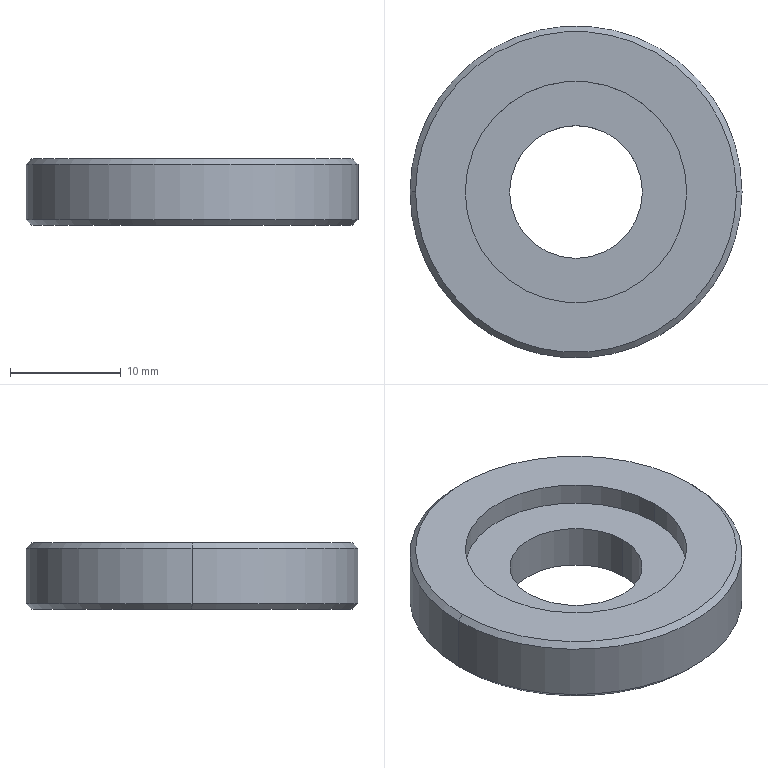Part | STEP file | PN_0100 Mount electronic clip blade | 1 solid | 13 faces | box 30 x 30 x 6 mm | volume 3137 mm3 | cylinder 6 | cone 4 | plane 3 | commonest cylinder face diameters 12 x2 20 x2 30 x2
STEP:
#1=CARTESIAN_POINT('',(0.,0.,0.));
#2=DIRECTION('',(0.,0.,1.));
#3=DIRECTION('',(1.,0.,0.));
#4=AXIS2_PLACEMENT_3D('',#1,#2,#3);
#5=CARTESIAN_POINT('',(14.5,0.,6.));
#6=VERTEX_POINT('',#5);
#7=CARTESIAN_POINT('',(-14.5,0.,6.));
#8=VERTEX_POINT('',#7);
#9=CARTESIAN_POINT('',(0.,0.,6.));
#10=DIRECTION('',(0.,0.,1.));
#11=DIRECTION('',(1.,0.,0.));
#12=AXIS2_PLACEMENT_3D('',#9,#10,#11);
#13=CIRCLE('',#12,14.5);
#14=CARTESIAN_POINT('',(0.,0.,6.));
#15=DIRECTION('',(0.,0.,-1.));
#16=DIRECTION('',(-1.,0.,0.));
#17=AXIS2_PLACEMENT_3D('',#14,#15,#16);
#18=CONICAL_SURFACE('',#17,14.5,0.7854);
#19=CARTESIAN_POINT('',(3.142,0.));
#20=DIRECTION('',(-1.,0.));
#21=VECTOR('',#20,1.);
#22=LINE('',#19,#21);
#23=(GEOMETRIC_REPRESENTATION_CONTEXT(2)PARAMETRIC_REPRESENTATION_CONTEXT()REPRESENTATION_CONTEXT('',''));
#24=DEFINITIONAL_REPRESENTATION('',(#22),#23);
#25=PCURVE('',#18,#24);
#26=CARTESIAN_POINT('',(0.,0.,6.));
#27=DIRECTION('',(0.,0.,1.));
#28=DIRECTION('',(1.,0.,0.));
#29=AXIS2_PLACEMENT_3D('',#26,#27,#28);
#30=PLANE('',#29);
#31=CARTESIAN_POINT('',(0.,0.));
#32=DIRECTION('',(1.,0.));
#33=AXIS2_PLACEMENT_2D('',#31,#32);
#34=CIRCLE('',#33,14.5);
#35=(GEOMETRIC_REPRESENTATION_CONTEXT(2)PARAMETRIC_REPRESENTATION_CONTEXT()REPRESENTATION_CONTEXT('',''));
#36=DEFINITIONAL_REPRESENTATION('',(#34),#35);
#37=PCURVE('',#30,#36);
#38=SURFACE_CURVE('',#13,(#25,#37),.PCURVE_S1.);
#39=EDGE_CURVE('',#6,#8,#38,.T.);
#40=ORIENTED_EDGE('',*,*,#39,.F.);
#41=CARTESIAN_POINT('',(15.,0.,5.5));
#42=VERTEX_POINT('',#41);
#43=CARTESIAN_POINT('',(14.5,0.,6.));
#44=DIRECTION('',(0.7071,0.,-0.7071));
#45=VECTOR('',#44,1.);
#46=LINE('',#43,#45);
#47=CARTESIAN_POINT('',(3.142,0.));
#48=DIRECTION('',(0.,1.));
#49=VECTOR('',#48,1.);
#50=LINE('',#47,#49);
#51=(GEOMETRIC_REPRESENTATION_CONTEXT(2)PARAMETRIC_REPRESENTATION_CONTEXT()REPRESENTATION_CONTEXT('',''));
#52=DEFINITIONAL_REPRESENTATION('',(#50),#51);
#53=PCURVE('',#18,#52);
#54=CARTESIAN_POINT('',(0.,0.,6.));
#55=DIRECTION('',(0.,0.,-1.));
#56=DIRECTION('',(-1.,0.,0.));
#57=AXIS2_PLACEMENT_3D('',#54,#55,#56);
#58=CONICAL_SURFACE('',#57,14.5,0.7854);
#59=CARTESIAN_POINT('',(3.142,0.));
#60=DIRECTION('',(0.,1.));
#61=VECTOR('',#60,1.);
#62=LINE('',#59,#61);
#63=(GEOMETRIC_REPRESENTATION_CONTEXT(2)PARAMETRIC_REPRESENTATION_CONTEXT()REPRESENTATION_CONTEXT('',''));
#64=DEFINITIONAL_REPRESENTATION('',(#62),#63);
#65=PCURVE('',#58,#64);
#66=SURFACE_CURVE('',#46,(#53,#65),.PCURVE_S1.);
#67=EDGE_CURVE('',#6,#42,#66,.T.);
#68=ORIENTED_EDGE('',*,*,#67,.T.);
#69=CARTESIAN_POINT('',(-15.,0.,5.5));
#70=VERTEX_POINT('',#69);
#71=CARTESIAN_POINT('',(0.,0.,5.5));
#72=DIRECTION('',(0.,0.,-1.));
#73=DIRECTION('',(1.,0.,0.));
#74=AXIS2_PLACEMENT_3D('',#71,#72,#73);
#75=CIRCLE('',#74,15.);
#76=CARTESIAN_POINT('',(-3.142,0.5));
#77=DIRECTION('',(1.,0.));
#78=VECTOR('',#77,1.);
#79=LINE('',#76,#78);
#80=(GEOMETRIC_REPRESENTATION_CONTEXT(2)PARAMETRIC_REPRESENTATION_CONTEXT()REPRESENTATION_CONTEXT('',''));
#81=DEFINITIONAL_REPRESENTATION('',(#79),#80);
#82=PCURVE('',#18,#81);
#83=CARTESIAN_POINT('',(0.,0.,6.));
#84=DIRECTION('',(0.,0.,-1.));
#85=DIRECTION('',(-1.,0.,0.));
#86=AXIS2_PLACEMENT_3D('',#83,#84,#85);
#87=CYLINDRICAL_SURFACE('',#86,15.);
#88=CARTESIAN_POINT('',(-3.142,0.5));
#89=DIRECTION('',(1.,0.));
#90=VECTOR('',#89,1.);
#91=LINE('',#88,#90);
#92=(GEOMETRIC_REPRESENTATION_CONTEXT(2)PARAMETRIC_REPRESENTATION_CONTEXT()REPRESENTATION_CONTEXT('',''));
#93=DEFINITIONAL_REPRESENTATION('',(#91),#92);
#94=PCURVE('',#87,#93);
#95=SURFACE_CURVE('',#75,(#82,#94),.PCURVE_S1.);
#96=EDGE_CURVE('',#70,#42,#95,.T.);
#97=ORIENTED_EDGE('',*,*,#96,.F.);
#98=CARTESIAN_POINT('',(-14.5,0.,6.));
#99=DIRECTION('',(-0.7071,0.,-0.7071));
#100=VECTOR('',#99,1.);
#101=LINE('',#98,#100);
#102=CARTESIAN_POINT('',(0.,0.));
#103=DIRECTION('',(0.,1.));
#104=VECTOR('',#103,1.);
#105=LINE('',#102,#104);
#106=(GEOMETRIC_REPRESENTATION_CONTEXT(2)PARAMETRIC_REPRESENTATION_CONTEXT()REPRESENTATION_CONTEXT('',''));
#107=DEFINITIONAL_REPRESENTATION('',(#105),#106);
#108=PCURVE('',#18,#107);
#109=CARTESIAN_POINT('',(6.283,0.));
#110=DIRECTION('',(0.,1.));
#111=VECTOR('',#110,1.);
#112=LINE('',#109,#111);
#113=(GEOMETRIC_REPRESENTATION_CONTEXT(2)PARAMETRIC_REPRESENTATION_CONTEXT()REPRESENTATION_CONTEXT('',''));
#114=DEFINITIONAL_REPRESENTATION('',(#112),#113);
#115=PCURVE('',#58,#114);
#116=SURFACE_CURVE('',#101,(#108,#115),.PCURVE_S1.);
#117=EDGE_CURVE('',#8,#70,#116,.T.);
#118=ORIENTED_EDGE('',*,*,#117,.F.);
#119=EDGE_LOOP('',(#40,#68,#97,#118));
#120=FACE_BOUND('',#119,.T.);
#121=ADVANCED_FACE('',(#120),#18,.T.);
#122=CARTESIAN_POINT('',(-14.5,0.,0.));
#123=VERTEX_POINT('',#122);
#124=CARTESIAN_POINT('',(14.5,0.,0.));
#125=VERTEX_POINT('',#124);
#126=CARTESIAN_POINT('',(0.,0.,0.));
#127=DIRECTION('',(0.,0.,-1.));
#128=DIRECTION('',(1.,0.,0.));
#129=AXIS2_PLACEMENT_3D('',#126,#127,#128);
#130=CIRCLE('',#129,14.5);
#131=CARTESIAN_POINT('',(0.,0.,0.5));
#132=DIRECTION('',(0.,0.,1.));
#133=DIRECTION('',(1.,0.,0.));
#134=AXIS2_PLACEMENT_3D('',#131,#132,#133);
#135=CONICAL_SURFACE('',#134,15.,0.7854);
#136=CARTESIAN_POINT('',(6.283,-0.5));
#137=DIRECTION('',(-1.,0.));
#138=VECTOR('',#137,1.);
#139=LINE('',#136,#138);
#140=(GEOMETRIC_REPRESENTATION_CONTEXT(2)PARAMETRIC_REPRESENTATION_CONTEXT()REPRESENTATION_CONTEXT('',''));
#141=DEFINITIONAL_REPRESENTATION('',(#139),#140);
#142=PCURVE('',#135,#141);
#143=CARTESIAN_POINT('',(0.,0.,0.));
#144=DIRECTION('',(0.,0.,1.));
#145=DIRECTION('',(1.,0.,0.));
#146=AXIS2_PLACEMENT_3D('',#143,#144,#145);
#147=PLANE('',#146);
#148=CARTESIAN_POINT('',(14.5,0.));
#149=CARTESIAN_POINT('',(14.5,-25.115));
#150=CARTESIAN_POINT('',(-7.25,-12.557));
#151=CARTESIAN_POINT('',(-29.,0.));
#152=CARTESIAN_POINT('',(-7.25,12.557));
#153=CARTESIAN_POINT('',(14.5,25.115));
#154=CARTESIAN_POINT('',(14.5,0.));
#155=(BOUNDED_CURVE()B_SPLINE_CURVE(2,(#148,#149,#150,#151,#152,#153,#154),.UNSPECIFIED.,.T.,.F.)B_SPLINE_CURVE_WITH_KNOTS((1,2,2,2,2,1),(-2.094,0.,2.094,4.189,6.283,8.378),.UNSPECIFIED.)CURVE()GEOMETRIC_REPRESENTATION_ITEM()RATIONAL_B_SPLINE_CURVE((1.,0.5,1.,0.5,1.,0.5,1.))REPRESENTATION_ITEM(''));
#156=(GEOMETRIC_REPRESENTATION_CONTEXT(2)PARAMETRIC_REPRESENTATION_CONTEXT()REPRESENTATION_CONTEXT('',''));
#157=DEFINITIONAL_REPRESENTATION('',(#155),#156);
#158=PCURVE('',#147,#157);
#159=SURFACE_CURVE('',#130,(#142,#158),.PCURVE_S1.);
#160=EDGE_CURVE('',#123,#125,#159,.T.);
#161=ORIENTED_EDGE('',*,*,#160,.F.);
#162=CARTESIAN_POINT('',(-15.,0.,0.5));
#163=VERTEX_POINT('',#162);
#164=CARTESIAN_POINT('',(-15.,0.,0.5));
#165=DIRECTION('',(-0.7071,0.,0.7071));
#166=VECTOR('',#165,1.);
#167=LINE('',#164,#166);
#168=CARTESIAN_POINT('',(3.142,0.));
#169=DIRECTION('',(0.,1.));
#170=VECTOR('',#169,1.);
#171=LINE('',#168,#170);
#172=(GEOMETRIC_REPRESENTATION_CONTEXT(2)PARAMETRIC_REPRESENTATION_CONTEXT()REPRESENTATION_CONTEXT('',''));
#173=DEFINITIONAL_REPRESENTATION('',(#171),#172);
#174=PCURVE('',#135,#173);
#175=CARTESIAN_POINT('',(0.,0.,0.5));
#176=DIRECTION('',(0.,0.,1.));
#177=DIRECTION('',(1.,0.,0.));
#178=AXIS2_PLACEMENT_3D('',#175,#176,#177);
#179=CONICAL_SURFACE('',#178,15.,0.7854);
#180=CARTESIAN_POINT('',(3.142,0.));
#181=DIRECTION('',(0.,1.));
#182=VECTOR('',#181,1.);
#183=LINE('',#180,#182);
#184=(GEOMETRIC_REPRESENTATION_CONTEXT(2)PARAMETRIC_REPRESENTATION_CONTEXT()REPRESENTATION_CONTEXT('',''));
#185=DEFINITIONAL_REPRESENTATION('',(#183),#184);
#186=PCURVE('',#179,#185);
#187=SURFACE_CURVE('',#167,(#174,#186),.PCURVE_S1.);
#188=EDGE_CURVE('',#123,#163,#187,.T.);
#189=ORIENTED_EDGE('',*,*,#188,.T.);
#190=CARTESIAN_POINT('',(15.,0.,0.5));
#191=VERTEX_POINT('',#190);
#192=CARTESIAN_POINT('',(0.,0.,0.5));
#193=DIRECTION('',(0.,0.,1.));
#194=DIRECTION('',(1.,0.,0.));
#195=AXIS2_PLACEMENT_3D('',#192,#193,#194);
#196=CIRCLE('',#195,15.);
#197=CARTESIAN_POINT('',(0.,0.));
#198=DIRECTION('',(1.,0.));
#199=VECTOR('',#198,1.);
#200=LINE('',#197,#199);
#201=(GEOMETRIC_REPRESENTATION_CONTEXT(2)PARAMETRIC_REPRESENTATION_CONTEXT()REPRESENTATION_CONTEXT('',''));
#202=DEFINITIONAL_REPRESENTATION('',(#200),#201);
#203=PCURVE('',#135,#202);
#204=CARTESIAN_POINT('',(3.142,5.5));
#205=DIRECTION('',(-1.,0.));
#206=VECTOR('',#205,1.);
#207=LINE('',#204,#206);
#208=(GEOMETRIC_REPRESENTATION_CONTEXT(2)PARAMETRIC_REPRESENTATION_CONTEXT()REPRESENTATION_CONTEXT('',''));
#209=DEFINITIONAL_REPRESENTATION('',(#207),#208);
#210=PCURVE('',#87,#209);
#211=SURFACE_CURVE('',#196,(#203,#210),.PCURVE_S1.);
#212=EDGE_CURVE('',#191,#163,#211,.T.);
#213=ORIENTED_EDGE('',*,*,#212,.F.);
#214=CARTESIAN_POINT('',(15.,0.,0.5));
#215=DIRECTION('',(0.7071,0.,0.7071));
#216=VECTOR('',#215,1.);
#217=LINE('',#214,#216);
#218=CARTESIAN_POINT('',(0.,0.));
#219=DIRECTION('',(0.,1.));
#220=VECTOR('',#219,1.);
#221=LINE('',#218,#220);
#222=(GEOMETRIC_REPRESENTATION_CONTEXT(2)PARAMETRIC_REPRESENTATION_CONTEXT()REPRESENTATION_CONTEXT('',''));
#223=DEFINITIONAL_REPRESENTATION('',(#221),#222);
#224=PCURVE('',#135,#223);
#225=CARTESIAN_POINT('',(6.283,0.));
#226=DIRECTION('',(0.,1.));
#227=VECTOR('',#226,1.);
#228=LINE('',#225,#227);
#229=(GEOMETRIC_REPRESENTATION_CONTEXT(2)PARAMETRIC_REPRESENTATION_CONTEXT()REPRESENTATION_CONTEXT('',''));
#230=DEFINITIONAL_REPRESENTATION('',(#228),#229);
#231=PCURVE('',#179,#230);
#232=SURFACE_CURVE('',#217,(#224,#231),.PCURVE_S1.);
#233=EDGE_CURVE('',#125,#191,#232,.T.);
#234=ORIENTED_EDGE('',*,*,#233,.F.);
#235=EDGE_LOOP('',(#161,#189,#213,#234));
#236=FACE_BOUND('',#235,.T.);
#237=ADVANCED_FACE('',(#236),#135,.T.);
#238=CARTESIAN_POINT('',(10.,0.,4.));
#239=VERTEX_POINT('',#238);
#240=CARTESIAN_POINT('',(10.,0.,6.));
#241=VERTEX_POINT('',#240);
#242=CARTESIAN_POINT('',(10.,0.,4.));
#243=DIRECTION('',(0.,0.,1.));
#244=VECTOR('',#243,1.);
#245=LINE('',#242,#244);
#246=CARTESIAN_POINT('',(0.,0.,4.));
#247=DIRECTION('',(0.,0.,1.));
#248=DIRECTION('',(1.,0.,0.));
#249=AXIS2_PLACEMENT_3D('',#246,#247,#248);
#250=CYLINDRICAL_SURFACE('',#249,10.);
#251=CARTESIAN_POINT('',(6.283,0.));
#252=DIRECTION('',(0.,1.));
#253=VECTOR('',#252,1.);
#254=LINE('',#251,#253);
#255=(GEOMETRIC_REPRESENTATION_CONTEXT(2)PARAMETRIC_REPRESENTATION_CONTEXT()REPRESENTATION_CONTEXT('',''));
#256=DEFINITIONAL_REPRESENTATION('',(#254),#255);
#257=PCURVE('',#250,#256);
#258=CARTESIAN_POINT('',(0.,0.,4.));
#259=DIRECTION('',(0.,0.,1.));
#260=DIRECTION('',(1.,0.,0.));
#261=AXIS2_PLACEMENT_3D('',#258,#259,#260);
#262=CYLINDRICAL_SURFACE('',#261,10.);
#263=CARTESIAN_POINT('',(0.,0.));
#264=DIRECTION('',(0.,1.));
#265=VECTOR('',#264,1.);
#266=LINE('',#263,#265);
#267=(GEOMETRIC_REPRESENTATION_CONTEXT(2)PARAMETRIC_REPRESENTATION_CONTEXT()REPRESENTATION_CONTEXT('',''));
#268=DEFINITIONAL_REPRESENTATION('',(#266),#267);
#269=PCURVE('',#262,#268);
#270=SURFACE_CURVE('',#245,(#257,#269),.PCURVE_S1.);
#271=EDGE_CURVE('',#239,#241,#270,.T.);
#272=ORIENTED_EDGE('',*,*,#271,.T.);
#273=CARTESIAN_POINT('',(-10.,0.,6.));
#274=VERTEX_POINT('',#273);
#275=CARTESIAN_POINT('',(0.,0.,6.));
#276=DIRECTION('',(0.,0.,1.));
#277=DIRECTION('',(1.,0.,0.));
#278=AXIS2_PLACEMENT_3D('',#275,#276,#277);
#279=CIRCLE('',#278,10.);
#280=CARTESIAN_POINT('',(0.,2.));
#281=DIRECTION('',(1.,0.));
#282=VECTOR('',#281,1.);
#283=LINE('',#280,#282);
#284=(GEOMETRIC_REPRESENTATION_CONTEXT(2)PARAMETRIC_REPRESENTATION_CONTEXT()REPRESENTATION_CONTEXT('',''));
#285=DEFINITIONAL_REPRESENTATION('',(#283),#284);
#286=PCURVE('',#250,#285);
#287=CARTESIAN_POINT('',(0.,0.));
#288=DIRECTION('',(1.,0.));
#289=AXIS2_PLACEMENT_2D('',#287,#288);
#290=CIRCLE('',#289,10.);
#291=(GEOMETRIC_REPRESENTATION_CONTEXT(2)PARAMETRIC_REPRESENTATION_CONTEXT()REPRESENTATION_CONTEXT('',''));
#292=DEFINITIONAL_REPRESENTATION('',(#290),#291);
#293=PCURVE('',#30,#292);
#294=SURFACE_CURVE('',#279,(#286,#293),.PCURVE_S1.);
#295=EDGE_CURVE('',#274,#241,#294,.T.);
#296=ORIENTED_EDGE('',*,*,#295,.F.);
#297=CARTESIAN_POINT('',(-10.,0.,4.));
#298=VERTEX_POINT('',#297);
#299=CARTESIAN_POINT('',(-10.,0.,4.));
#300=DIRECTION('',(0.,0.,1.));
#301=VECTOR('',#300,1.);
#302=LINE('',#299,#301);
#303=CARTESIAN_POINT('',(3.142,0.));
#304=DIRECTION('',(0.,1.));
#305=VECTOR('',#304,1.);
#306=LINE('',#303,#305);
#307=(GEOMETRIC_REPRESENTATION_CONTEXT(2)PARAMETRIC_REPRESENTATION_CONTEXT()REPRESENTATION_CONTEXT('',''));
#308=DEFINITIONAL_REPRESENTATION('',(#306),#307);
#309=PCURVE('',#250,#308);
#310=CARTESIAN_POINT('',(3.142,0.));
#311=DIRECTION('',(0.,1.));
#312=VECTOR('',#311,1.);
#313=LINE('',#310,#312);
#314=(GEOMETRIC_REPRESENTATION_CONTEXT(2)PARAMETRIC_REPRESENTATION_CONTEXT()REPRESENTATION_CONTEXT('',''));
#315=DEFINITIONAL_REPRESENTATION('',(#313),#314);
#316=PCURVE('',#262,#315);
#317=SURFACE_CURVE('',#302,(#309,#316),.PCURVE_S1.);
#318=EDGE_CURVE('',#298,#274,#317,.T.);
#319=ORIENTED_EDGE('',*,*,#318,.F.);
#320=CARTESIAN_POINT('',(0.,0.,4.));
#321=DIRECTION('',(0.,0.,1.));
#322=DIRECTION('',(1.,0.,0.));
#323=AXIS2_PLACEMENT_3D('',#320,#321,#322);
#324=CIRCLE('',#323,10.);
#325=CARTESIAN_POINT('',(0.,0.));
#326=DIRECTION('',(1.,0.));
#327=VECTOR('',#326,1.);
#328=LINE('',#325,#327);
#329=(GEOMETRIC_REPRESENTATION_CONTEXT(2)PARAMETRIC_REPRESENTATION_CONTEXT()REPRESENTATION_CONTEXT('',''));
#330=DEFINITIONAL_REPRESENTATION('',(#328),#329);
#331=PCURVE('',#250,#330);
#332=CARTESIAN_POINT('',(0.,0.,4.));
#333=DIRECTION('',(0.,0.,1.));
#334=DIRECTION('',(1.,0.,0.));
#335=AXIS2_PLACEMENT_3D('',#332,#333,#334);
#336=PLANE('',#335);
#337=CARTESIAN_POINT('',(0.,0.));
#338=DIRECTION('',(1.,0.));
#339=AXIS2_PLACEMENT_2D('',#337,#338);
#340=CIRCLE('',#339,10.);
#341=(GEOMETRIC_REPRESENTATION_CONTEXT(2)PARAMETRIC_REPRESENTATION_CONTEXT()REPRESENTATION_CONTEXT('',''));
#342=DEFINITIONAL_REPRESENTATION('',(#340),#341);
#343=PCURVE('',#336,#342);
#344=SURFACE_CURVE('',#324,(#331,#343),.PCURVE_S1.);
#345=EDGE_CURVE('',#298,#239,#344,.T.);
#346=ORIENTED_EDGE('',*,*,#345,.T.);
#347=EDGE_LOOP('',(#272,#296,#319,#346));
#348=FACE_BOUND('',#347,.F.);
#349=ADVANCED_FACE('',(#348),#250,.F.);
#350=ORIENTED_EDGE('',*,*,#96,.T.);
#351=CARTESIAN_POINT('',(15.,0.,6.));
#352=DIRECTION('',(0.,0.,-1.));
#353=VECTOR('',#352,1.);
#354=LINE('',#351,#353);
#355=CARTESIAN_POINT('',(3.142,0.));
#356=DIRECTION('',(0.,1.));
#357=VECTOR('',#356,1.);
#358=LINE('',#355,#357);
#359=(GEOMETRIC_REPRESENTATION_CONTEXT(2)PARAMETRIC_REPRESENTATION_CONTEXT()REPRESENTATION_CONTEXT('',''));
#360=DEFINITIONAL_REPRESENTATION('',(#358),#359);
#361=PCURVE('',#87,#360);
#362=CARTESIAN_POINT('',(0.,0.,6.));
#363=DIRECTION('',(0.,0.,-1.));
#364=DIRECTION('',(-1.,0.,0.));
#365=AXIS2_PLACEMENT_3D('',#362,#363,#364);
#366=CYLINDRICAL_SURFACE('',#365,15.);
#367=CARTESIAN_POINT('',(3.142,0.));
#368=DIRECTION('',(0.,1.));
#369=VECTOR('',#368,1.);
#370=LINE('',#367,#369);
#371=(GEOMETRIC_REPRESENTATION_CONTEXT(2)PARAMETRIC_REPRESENTATION_CONTEXT()REPRESENTATION_CONTEXT('',''));
#372=DEFINITIONAL_REPRESENTATION('',(#370),#371);
#373=PCURVE('',#366,#372);
#374=SURFACE_CURVE('',#354,(#361,#373),.PCURVE_S1.);
#375=EDGE_CURVE('',#42,#191,#374,.T.);
#376=ORIENTED_EDGE('',*,*,#375,.T.);
#377=ORIENTED_EDGE('',*,*,#212,.T.);
#378=CARTESIAN_POINT('',(-15.,0.,6.));
#379=DIRECTION('',(0.,0.,-1.));
#380=VECTOR('',#379,1.);
#381=LINE('',#378,#380);
#382=CARTESIAN_POINT('',(0.,0.));
#383=DIRECTION('',(0.,1.));
#384=VECTOR('',#383,1.);
#385=LINE('',#382,#384);
#386=(GEOMETRIC_REPRESENTATION_CONTEXT(2)PARAMETRIC_REPRESENTATION_CONTEXT()REPRESENTATION_CONTEXT('',''));
#387=DEFINITIONAL_REPRESENTATION('',(#385),#386);
#388=PCURVE('',#87,#387);
#389=CARTESIAN_POINT('',(6.283,0.));
#390=DIRECTION('',(0.,1.));
#391=VECTOR('',#390,1.);
#392=LINE('',#389,#391);
#393=(GEOMETRIC_REPRESENTATION_CONTEXT(2)PARAMETRIC_REPRESENTATION_CONTEXT()REPRESENTATION_CONTEXT('',''));
#394=DEFINITIONAL_REPRESENTATION('',(#392),#393);
#395=PCURVE('',#366,#394);
#396=SURFACE_CURVE('',#381,(#388,#395),.PCURVE_S1.);
#397=EDGE_CURVE('',#70,#163,#396,.T.);
#398=ORIENTED_EDGE('',*,*,#397,.F.);
#399=EDGE_LOOP('',(#350,#376,#377,#398));
#400=FACE_BOUND('',#399,.T.);
#401=ADVANCED_FACE('',(#400),#87,.T.);
#402=CARTESIAN_POINT('',(-6.,0.,4.));
#403=VERTEX_POINT('',#402);
#404=CARTESIAN_POINT('',(-6.,0.,0.));
#405=VERTEX_POINT('',#404);
#406=CARTESIAN_POINT('',(-6.,0.,6.));
#407=DIRECTION('',(0.,0.,-1.));
#408=VECTOR('',#407,1.);
#409=LINE('',#406,#408);
#410=CARTESIAN_POINT('',(0.,0.,6.));
#411=DIRECTION('',(0.,0.,-1.));
#412=DIRECTION('',(-1.,0.,0.));
#413=AXIS2_PLACEMENT_3D('',#410,#411,#412);
#414=CYLINDRICAL_SURFACE('',#413,6.);
#415=CARTESIAN_POINT('',(6.283,0.));
#416=DIRECTION('',(0.,1.));
#417=VECTOR('',#416,1.);
#418=LINE('',#415,#417);
#419=(GEOMETRIC_REPRESENTATION_CONTEXT(2)PARAMETRIC_REPRESENTATION_CONTEXT()REPRESENTATION_CONTEXT('',''));
#420=DEFINITIONAL_REPRESENTATION('',(#418),#419);
#421=PCURVE('',#414,#420);
#422=CARTESIAN_POINT('',(0.,0.,6.));
#423=DIRECTION('',(0.,0.,-1.));
#424=DIRECTION('',(-1.,0.,0.));
#425=AXIS2_PLACEMENT_3D('',#422,#423,#424);
#426=CYLINDRICAL_SURFACE('',#425,6.);
#427=CARTESIAN_POINT('',(0.,0.));
#428=DIRECTION('',(0.,1.));
#429=VECTOR('',#428,1.);
#430=LINE('',#427,#429);
#431=(GEOMETRIC_REPRESENTATION_CONTEXT(2)PARAMETRIC_REPRESENTATION_CONTEXT()REPRESENTATION_CONTEXT('',''));
#432=DEFINITIONAL_REPRESENTATION('',(#430),#431);
#433=PCURVE('',#426,#432);
#434=SURFACE_CURVE('',#409,(#421,#433),.PCURVE_S1.);
#435=EDGE_CURVE('',#403,#405,#434,.T.);
#436=ORIENTED_EDGE('',*,*,#435,.T.);
#437=CARTESIAN_POINT('',(6.,0.,0.));
#438=VERTEX_POINT('',#437);
#439=CARTESIAN_POINT('',(0.,0.,0.));
#440=DIRECTION('',(0.,0.,1.));
#441=DIRECTION('',(1.,0.,0.));
#442=AXIS2_PLACEMENT_3D('',#439,#440,#441);
#443=CIRCLE('',#442,6.);
#444=CARTESIAN_POINT('',(9.425,6.));
#445=DIRECTION('',(-1.,0.));
#446=VECTOR('',#445,1.);
#447=LINE('',#444,#446);
#448=(GEOMETRIC_REPRESENTATION_CONTEXT(2)PARAMETRIC_REPRESENTATION_CONTEXT()REPRESENTATION_CONTEXT('',''));
#449=DEFINITIONAL_REPRESENTATION('',(#447),#448);
#450=PCURVE('',#414,#449);
#451=CARTESIAN_POINT('',(0.,0.));
#452=DIRECTION('',(1.,0.));
#453=AXIS2_PLACEMENT_2D('',#451,#452);
#454=CIRCLE('',#453,6.);
#455=(GEOMETRIC_REPRESENTATION_CONTEXT(2)PARAMETRIC_REPRESENTATION_CONTEXT()REPRESENTATION_CONTEXT('',''));
#456=DEFINITIONAL_REPRESENTATION('',(#454),#455);
#457=PCURVE('',#147,#456);
#458=SURFACE_CURVE('',#443,(#450,#457),.PCURVE_S1.);
#459=EDGE_CURVE('',#405,#438,#458,.T.);
#460=ORIENTED_EDGE('',*,*,#459,.T.);
#461=CARTESIAN_POINT('',(6.,0.,4.));
#462=VERTEX_POINT('',#461);
#463=CARTESIAN_POINT('',(6.,0.,6.));
#464=DIRECTION('',(0.,0.,-1.));
#465=VECTOR('',#464,1.);
#466=LINE('',#463,#465);
#467=CARTESIAN_POINT('',(3.142,0.));
#468=DIRECTION('',(0.,1.));
#469=VECTOR('',#468,1.);
#470=LINE('',#467,#469);
#471=(GEOMETRIC_REPRESENTATION_CONTEXT(2)PARAMETRIC_REPRESENTATION_CONTEXT()REPRESENTATION_CONTEXT('',''));
#472=DEFINITIONAL_REPRESENTATION('',(#470),#471);
#473=PCURVE('',#414,#472);
#474=CARTESIAN_POINT('',(3.142,0.));
#475=DIRECTION('',(0.,1.));
#476=VECTOR('',#475,1.);
#477=LINE('',#474,#476);
#478=(GEOMETRIC_REPRESENTATION_CONTEXT(2)PARAMETRIC_REPRESENTATION_CONTEXT()REPRESENTATION_CONTEXT('',''));
#479=DEFINITIONAL_REPRESENTATION('',(#477),#478);
#480=PCURVE('',#426,#479);
#481=SURFACE_CURVE('',#466,(#473,#480),.PCURVE_S1.);
#482=EDGE_CURVE('',#462,#438,#481,.T.);
#483=ORIENTED_EDGE('',*,*,#482,.F.);
#484=CARTESIAN_POINT('',(0.,0.,4.));
#485=DIRECTION('',(0.,0.,1.));
#486=DIRECTION('',(1.,0.,0.));
#487=AXIS2_PLACEMENT_3D('',#484,#485,#486);
#488=CIRCLE('',#487,6.);
#489=CARTESIAN_POINT('',(9.425,2.));
#490=DIRECTION('',(-1.,0.));
#491=VECTOR('',#490,1.);
#492=LINE('',#489,#491);
#493=(GEOMETRIC_REPRESENTATION_CONTEXT(2)PARAMETRIC_REPRESENTATION_CONTEXT()REPRESENTATION_CONTEXT('',''));
#494=DEFINITIONAL_REPRESENTATION('',(#492),#493);
#495=PCURVE('',#414,#494);
#496=CARTESIAN_POINT('',(0.,0.));
#497=DIRECTION('',(1.,0.));
#498=AXIS2_PLACEMENT_2D('',#496,#497);
#499=CIRCLE('',#498,6.);
#500=(GEOMETRIC_REPRESENTATION_CONTEXT(2)PARAMETRIC_REPRESENTATION_CONTEXT()REPRESENTATION_CONTEXT('',''));
#501=DEFINITIONAL_REPRESENTATION('',(#499),#500);
#502=PCURVE('',#336,#501);
#503=SURFACE_CURVE('',#488,(#495,#502),.PCURVE_S1.);
#504=EDGE_CURVE('',#403,#462,#503,.T.);
#505=ORIENTED_EDGE('',*,*,#504,.F.);
#506=EDGE_LOOP('',(#436,#460,#483,#505));
#507=FACE_BOUND('',#506,.F.);
#508=ADVANCED_FACE('',(#507),#414,.F.);
#509=CARTESIAN_POINT('',(0.,0.,0.));
#510=DIRECTION('',(0.,0.,1.));
#511=DIRECTION('',(1.,0.,0.));
#512=AXIS2_PLACEMENT_3D('',#509,#510,#511);
#513=CIRCLE('',#512,6.);
#514=CARTESIAN_POINT('',(3.142,6.));
#515=DIRECTION('',(-1.,0.));
#516=VECTOR('',#515,1.);
#517=LINE('',#514,#516);
#518=(GEOMETRIC_REPRESENTATION_CONTEXT(2)PARAMETRIC_REPRESENTATION_CONTEXT()REPRESENTATION_CONTEXT('',''));
#519=DEFINITIONAL_REPRESENTATION('',(#517),#518);
#520=PCURVE('',#426,#519);
#521=CARTESIAN_POINT('',(0.,0.));
#522=DIRECTION('',(1.,0.));
#523=AXIS2_PLACEMENT_2D('',#521,#522);
#524=CIRCLE('',#523,6.);
#525=(GEOMETRIC_REPRESENTATION_CONTEXT(2)PARAMETRIC_REPRESENTATION_CONTEXT()REPRESENTATION_CONTEXT('',''));
#526=DEFINITIONAL_REPRESENTATION('',(#524),#525);
#527=PCURVE('',#147,#526);
#528=SURFACE_CURVE('',#513,(#520,#527),.PCURVE_S1.);
#529=EDGE_CURVE('',#438,#405,#528,.T.);
#530=ORIENTED_EDGE('',*,*,#529,.T.);
#531=ORIENTED_EDGE('',*,*,#435,.F.);
#532=CARTESIAN_POINT('',(0.,0.,4.));
#533=DIRECTION('',(0.,0.,1.));
#534=DIRECTION('',(1.,0.,0.));
#535=AXIS2_PLACEMENT_3D('',#532,#533,#534);
#536=CIRCLE('',#535,6.);
#537=CARTESIAN_POINT('',(3.142,2.));
#538=DIRECTION('',(-1.,0.));
#539=VECTOR('',#538,1.);
#540=LINE('',#537,#539);
#541=(GEOMETRIC_REPRESENTATION_CONTEXT(2)PARAMETRIC_REPRESENTATION_CONTEXT()REPRESENTATION_CONTEXT('',''));
#542=DEFINITIONAL_REPRESENTATION('',(#540),#541);
#543=PCURVE('',#426,#542);
#544=CARTESIAN_POINT('',(0.,0.));
#545=DIRECTION('',(1.,0.));
#546=AXIS2_PLACEMENT_2D('',#544,#545);
#547=CIRCLE('',#546,6.);
#548=(GEOMETRIC_REPRESENTATION_CONTEXT(2)PARAMETRIC_REPRESENTATION_CONTEXT()REPRESENTATION_CONTEXT('',''));
#549=DEFINITIONAL_REPRESENTATION('',(#547),#548);
#550=PCURVE('',#336,#549);
#551=SURFACE_CURVE('',#536,(#543,#550),.PCURVE_S1.);
#552=EDGE_CURVE('',#462,#403,#551,.T.);
#553=ORIENTED_EDGE('',*,*,#552,.F.);
#554=ORIENTED_EDGE('',*,*,#482,.T.);
#555=EDGE_LOOP('',(#530,#531,#553,#554));
#556=FACE_BOUND('',#555,.F.);
#557=ADVANCED_FACE('',(#556),#426,.F.);
#558=CARTESIAN_POINT('',(0.,0.,6.));
#559=DIRECTION('',(0.,0.,1.));
#560=DIRECTION('',(1.,0.,0.));
#561=AXIS2_PLACEMENT_3D('',#558,#559,#560);
#562=CIRCLE('',#561,14.5);
#563=CARTESIAN_POINT('',(0.,0.));
#564=DIRECTION('',(1.,0.));
#565=AXIS2_PLACEMENT_2D('',#563,#564);
#566=CIRCLE('',#565,14.5);
#567=(GEOMETRIC_REPRESENTATION_CONTEXT(2)PARAMETRIC_REPRESENTATION_CONTEXT()REPRESENTATION_CONTEXT('',''));
#568=DEFINITIONAL_REPRESENTATION('',(#566),#567);
#569=PCURVE('',#30,#568);
#570=CARTESIAN_POINT('',(9.425,0.));
#571=DIRECTION('',(-1.,0.));
#572=VECTOR('',#571,1.);
#573=LINE('',#570,#572);
#574=(GEOMETRIC_REPRESENTATION_CONTEXT(2)PARAMETRIC_REPRESENTATION_CONTEXT()REPRESENTATION_CONTEXT('',''));
#575=DEFINITIONAL_REPRESENTATION('',(#573),#574);
#576=PCURVE('',#58,#575);
#577=SURFACE_CURVE('',#562,(#569,#576),.PCURVE_S1.);
#578=EDGE_CURVE('',#8,#6,#577,.T.);
#579=ORIENTED_EDGE('',*,*,#578,.T.);
#580=ORIENTED_EDGE('',*,*,#39,.T.);
#581=EDGE_LOOP('',(#579,#580));
#582=FACE_BOUND('',#581,.T.);
#583=CARTESIAN_POINT('',(0.,0.,6.));
#584=DIRECTION('',(0.,0.,1.));
#585=DIRECTION('',(1.,0.,0.));
#586=AXIS2_PLACEMENT_3D('',#583,#584,#585);
#587=CIRCLE('',#586,10.);
#588=CARTESIAN_POINT('',(0.,0.));
#589=DIRECTION('',(1.,0.));
#590=AXIS2_PLACEMENT_2D('',#588,#589);
#591=CIRCLE('',#590,10.);
#592=(GEOMETRIC_REPRESENTATION_CONTEXT(2)PARAMETRIC_REPRESENTATION_CONTEXT()REPRESENTATION_CONTEXT('',''));
#593=DEFINITIONAL_REPRESENTATION('',(#591),#592);
#594=PCURVE('',#30,#593);
#595=CARTESIAN_POINT('',(0.,2.));
#596=DIRECTION('',(1.,0.));
#597=VECTOR('',#596,1.);
#598=LINE('',#595,#597);
#599=(GEOMETRIC_REPRESENTATION_CONTEXT(2)PARAMETRIC_REPRESENTATION_CONTEXT()REPRESENTATION_CONTEXT('',''));
#600=DEFINITIONAL_REPRESENTATION('',(#598),#599);
#601=PCURVE('',#262,#600);
#602=SURFACE_CURVE('',#587,(#594,#601),.PCURVE_S1.);
#603=EDGE_CURVE('',#241,#274,#602,.T.);
#604=ORIENTED_EDGE('',*,*,#603,.F.);
#605=ORIENTED_EDGE('',*,*,#295,.F.);
#606=EDGE_LOOP('',(#604,#605));
#607=FACE_BOUND('',#606,.T.);
#608=ADVANCED_FACE('',(#582,#607),#30,.T.);
#609=CARTESIAN_POINT('',(0.,0.,0.));
#610=DIRECTION('',(0.,0.,-1.));
#611=DIRECTION('',(1.,0.,0.));
#612=AXIS2_PLACEMENT_3D('',#609,#610,#611);
#613=CIRCLE('',#612,14.5);
#614=CARTESIAN_POINT('',(14.5,0.));
#615=CARTESIAN_POINT('',(14.5,-25.115));
#616=CARTESIAN_POINT('',(-7.25,-12.557));
#617=CARTESIAN_POINT('',(-29.,0.));
#618=CARTESIAN_POINT('',(-7.25,12.557));
#619=CARTESIAN_POINT('',(14.5,25.115));
#620=CARTESIAN_POINT('',(14.5,0.));
#621=(BOUNDED_CURVE()B_SPLINE_CURVE(2,(#614,#615,#616,#617,#618,#619,#620),.UNSPECIFIED.,.T.,.F.)B_SPLINE_CURVE_WITH_KNOTS((1,2,2,2,2,1),(-2.094,0.,2.094,4.189,6.283,8.378),.UNSPECIFIED.)CURVE()GEOMETRIC_REPRESENTATION_ITEM()RATIONAL_B_SPLINE_CURVE((1.,0.5,1.,0.5,1.,0.5,1.))REPRESENTATION_ITEM(''));
#622=(GEOMETRIC_REPRESENTATION_CONTEXT(2)PARAMETRIC_REPRESENTATION_CONTEXT()REPRESENTATION_CONTEXT('',''));
#623=DEFINITIONAL_REPRESENTATION('',(#621),#622);
#624=PCURVE('',#147,#623);
#625=CARTESIAN_POINT('',(6.283,-0.5));
#626=DIRECTION('',(-1.,0.));
#627=VECTOR('',#626,1.);
#628=LINE('',#625,#627);
#629=(GEOMETRIC_REPRESENTATION_CONTEXT(2)PARAMETRIC_REPRESENTATION_CONTEXT()REPRESENTATION_CONTEXT('',''));
#630=DEFINITIONAL_REPRESENTATION('',(#628),#629);
#631=PCURVE('',#179,#630);
#632=SURFACE_CURVE('',#613,(#624,#631),.PCURVE_S1.);
#633=EDGE_CURVE('',#125,#123,#632,.T.);
#634=ORIENTED_EDGE('',*,*,#633,.T.);
#635=ORIENTED_EDGE('',*,*,#160,.T.);
#636=EDGE_LOOP('',(#634,#635));
#637=FACE_BOUND('',#636,.T.);
#638=ORIENTED_EDGE('',*,*,#459,.T.);
#639=ORIENTED_EDGE('',*,*,#529,.T.);
#640=EDGE_LOOP('',(#638,#639));
#641=FACE_BOUND('',#640,.T.);
#642=ADVANCED_FACE('',(#637,#641),#147,.F.);
#643=ORIENTED_EDGE('',*,*,#375,.F.);
#644=CARTESIAN_POINT('',(0.,0.,5.5));
#645=DIRECTION('',(0.,0.,-1.));
#646=DIRECTION('',(1.,0.,0.));
#647=AXIS2_PLACEMENT_3D('',#644,#645,#646);
#648=CIRCLE('',#647,15.);
#649=CARTESIAN_POINT('',(3.142,0.5));
#650=DIRECTION('',(1.,0.));
#651=VECTOR('',#650,1.);
#652=LINE('',#649,#651);
#653=(GEOMETRIC_REPRESENTATION_CONTEXT(2)PARAMETRIC_REPRESENTATION_CONTEXT()REPRESENTATION_CONTEXT('',''));
#654=DEFINITIONAL_REPRESENTATION('',(#652),#653);
#655=PCURVE('',#366,#654);
#656=CARTESIAN_POINT('',(3.142,0.5));
#657=DIRECTION('',(1.,0.));
#658=VECTOR('',#657,1.);
#659=LINE('',#656,#658);
#660=(GEOMETRIC_REPRESENTATION_CONTEXT(2)PARAMETRIC_REPRESENTATION_CONTEXT()REPRESENTATION_CONTEXT('',''));
#661=DEFINITIONAL_REPRESENTATION('',(#659),#660);
#662=PCURVE('',#58,#661);
#663=SURFACE_CURVE('',#648,(#655,#662),.PCURVE_S1.);
#664=EDGE_CURVE('',#42,#70,#663,.T.);
#665=ORIENTED_EDGE('',*,*,#664,.T.);
#666=ORIENTED_EDGE('',*,*,#397,.T.);
#667=CARTESIAN_POINT('',(0.,0.,0.5));
#668=DIRECTION('',(0.,0.,1.));
#669=DIRECTION('',(1.,0.,0.));
#670=AXIS2_PLACEMENT_3D('',#667,#668,#669);
#671=CIRCLE('',#670,15.);
#672=CARTESIAN_POINT('',(9.425,5.5));
#673=DIRECTION('',(-1.,0.));
#674=VECTOR('',#673,1.);
#675=LINE('',#672,#674);
#676=(GEOMETRIC_REPRESENTATION_CONTEXT(2)PARAMETRIC_REPRESENTATION_CONTEXT()REPRESENTATION_CONTEXT('',''));
#677=DEFINITIONAL_REPRESENTATION('',(#675),#676);
#678=PCURVE('',#366,#677);
#679=CARTESIAN_POINT('',(0.,0.));
#680=DIRECTION('',(1.,0.));
#681=VECTOR('',#680,1.);
#682=LINE('',#679,#681);
#683=(GEOMETRIC_REPRESENTATION_CONTEXT(2)PARAMETRIC_REPRESENTATION_CONTEXT()REPRESENTATION_CONTEXT('',''));
#684=DEFINITIONAL_REPRESENTATION('',(#682),#683);
#685=PCURVE('',#179,#684);
#686=SURFACE_CURVE('',#671,(#678,#685),.PCURVE_S1.);
#687=EDGE_CURVE('',#163,#191,#686,.T.);
#688=ORIENTED_EDGE('',*,*,#687,.T.);
#689=EDGE_LOOP('',(#643,#665,#666,#688));
#690=FACE_BOUND('',#689,.T.);
#691=ADVANCED_FACE('',(#690),#366,.T.);
#692=ORIENTED_EDGE('',*,*,#603,.F.);
#693=ORIENTED_EDGE('',*,*,#271,.F.);
#694=CARTESIAN_POINT('',(0.,0.,4.));
#695=DIRECTION('',(0.,0.,1.));
#696=DIRECTION('',(1.,0.,0.));
#697=AXIS2_PLACEMENT_3D('',#694,#695,#696);
#698=CIRCLE('',#697,10.);
#699=CARTESIAN_POINT('',(0.,0.));
#700=DIRECTION('',(1.,0.));
#701=VECTOR('',#700,1.);
#702=LINE('',#699,#701);
#703=(GEOMETRIC_REPRESENTATION_CONTEXT(2)PARAMETRIC_REPRESENTATION_CONTEXT()REPRESENTATION_CONTEXT('',''));
#704=DEFINITIONAL_REPRESENTATION('',(#702),#703);
#705=PCURVE('',#262,#704);
#706=CARTESIAN_POINT('',(0.,0.));
#707=DIRECTION('',(1.,0.));
#708=AXIS2_PLACEMENT_2D('',#706,#707);
#709=CIRCLE('',#708,10.);
#710=(GEOMETRIC_REPRESENTATION_CONTEXT(2)PARAMETRIC_REPRESENTATION_CONTEXT()REPRESENTATION_CONTEXT('',''));
#711=DEFINITIONAL_REPRESENTATION('',(#709),#710);
#712=PCURVE('',#336,#711);
#713=SURFACE_CURVE('',#698,(#705,#712),.PCURVE_S1.);
#714=EDGE_CURVE('',#239,#298,#713,.T.);
#715=ORIENTED_EDGE('',*,*,#714,.T.);
#716=ORIENTED_EDGE('',*,*,#318,.T.);
#717=EDGE_LOOP('',(#692,#693,#715,#716));
#718=FACE_BOUND('',#717,.F.);
#719=ADVANCED_FACE('',(#718),#262,.F.);
#720=ORIENTED_EDGE('',*,*,#504,.F.);
#721=ORIENTED_EDGE('',*,*,#552,.F.);
#722=EDGE_LOOP('',(#720,#721));
#723=FACE_BOUND('',#722,.T.);
#724=ORIENTED_EDGE('',*,*,#714,.T.);
#725=ORIENTED_EDGE('',*,*,#345,.T.);
#726=EDGE_LOOP('',(#724,#725));
#727=FACE_BOUND('',#726,.T.);
#728=ADVANCED_FACE('',(#723,#727),#336,.T.);
#729=ORIENTED_EDGE('',*,*,#188,.F.);
#730=ORIENTED_EDGE('',*,*,#633,.F.);
#731=ORIENTED_EDGE('',*,*,#233,.T.);
#732=ORIENTED_EDGE('',*,*,#687,.F.);
#733=EDGE_LOOP('',(#729,#730,#731,#732));
#734=FACE_BOUND('',#733,.T.);
#735=ADVANCED_FACE('',(#734),#179,.T.);
#736=ORIENTED_EDGE('',*,*,#67,.F.);
#737=ORIENTED_EDGE('',*,*,#578,.F.);
#738=ORIENTED_EDGE('',*,*,#117,.T.);
#739=ORIENTED_EDGE('',*,*,#664,.F.);
#740=EDGE_LOOP('',(#736,#737,#738,#739));
#741=FACE_BOUND('',#740,.T.);
#742=ADVANCED_FACE('',(#741),#58,.T.);
#743=CLOSED_SHELL('',(#121,#237,#349,#401,#508,#557,#608,#642,#691,#719,#728,#735,#742));
#744=MANIFOLD_SOLID_BREP('',#743);
#745=(LENGTH_UNIT()NAMED_UNIT(*)SI_UNIT(.MILLI.,.METRE.));
#746=UNCERTAINTY_MEASURE_WITH_UNIT(LENGTH_MEASURE(0.0000001),#745,'','');
#747=(NAMED_UNIT(*)PLANE_ANGLE_UNIT()SI_UNIT($,.RADIAN.));
#748=(NAMED_UNIT(*)SI_UNIT($,.STERADIAN.)SOLID_ANGLE_UNIT());
#749=(GEOMETRIC_REPRESENTATION_CONTEXT(3)GLOBAL_UNCERTAINTY_ASSIGNED_CONTEXT((#746))GLOBAL_UNIT_ASSIGNED_CONTEXT((#745,#747,#748))REPRESENTATION_CONTEXT('',''));
#750=ADVANCED_BREP_SHAPE_REPRESENTATION('',(#4,#744),#749);